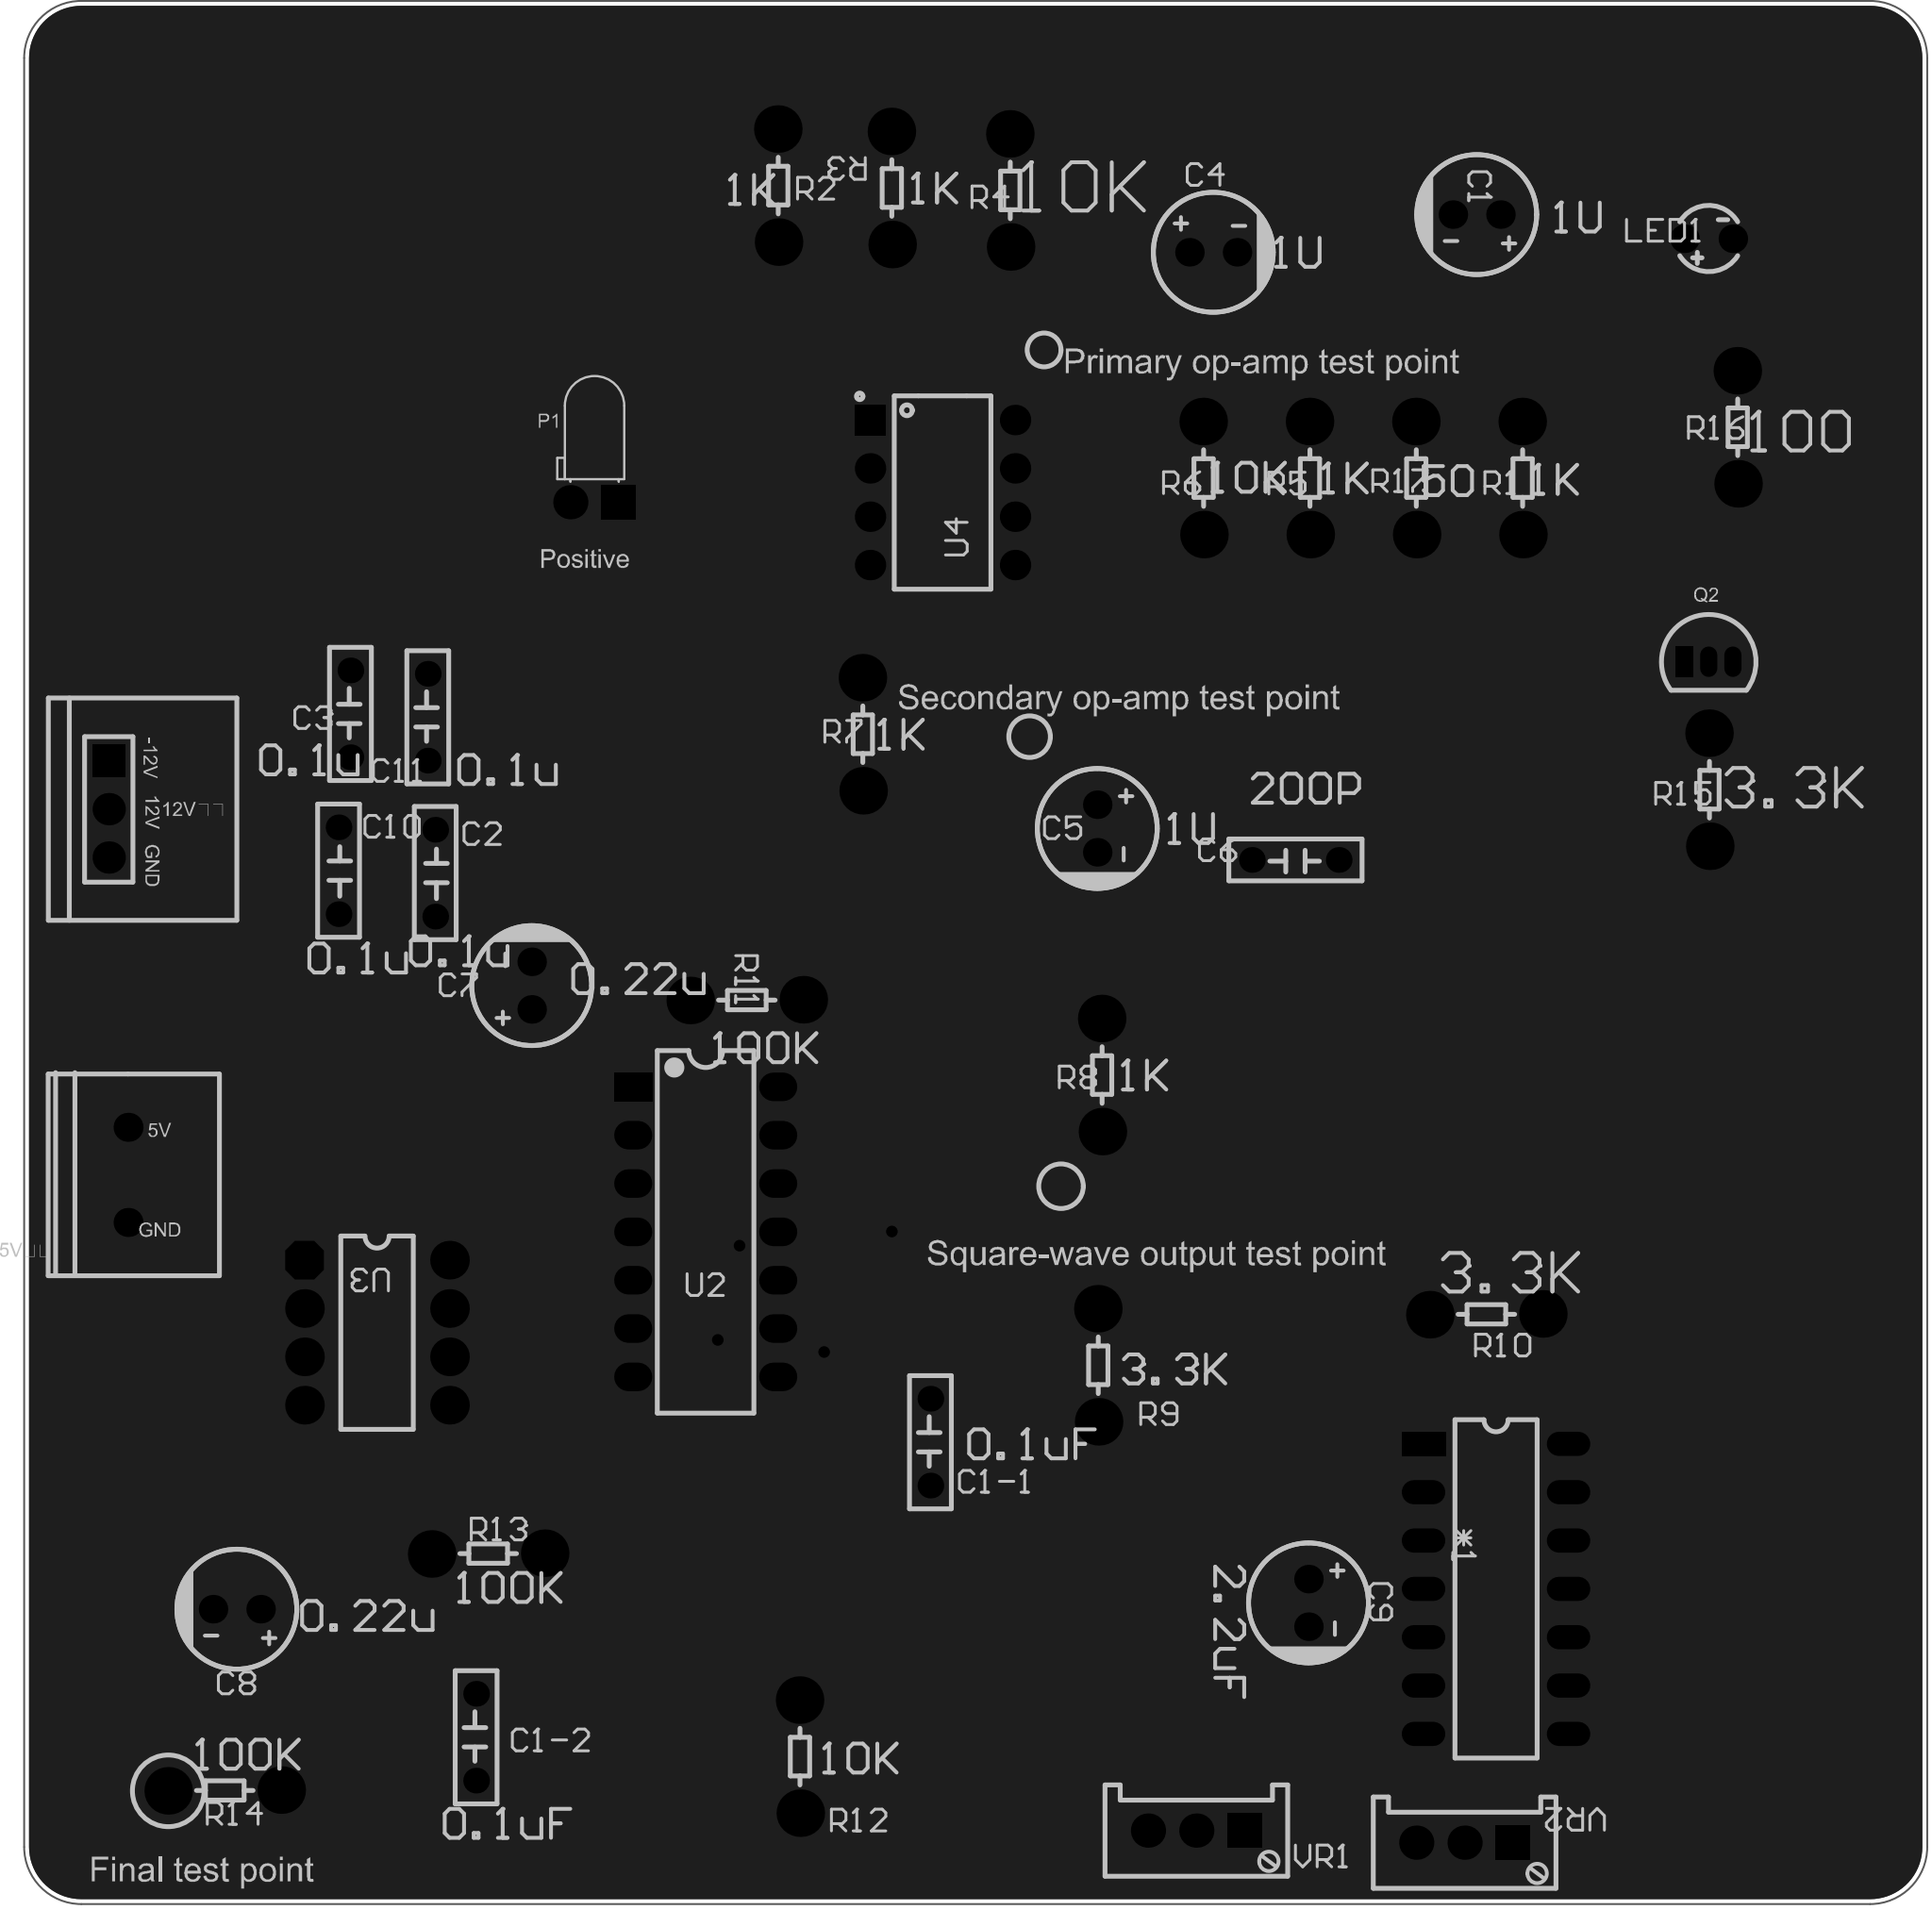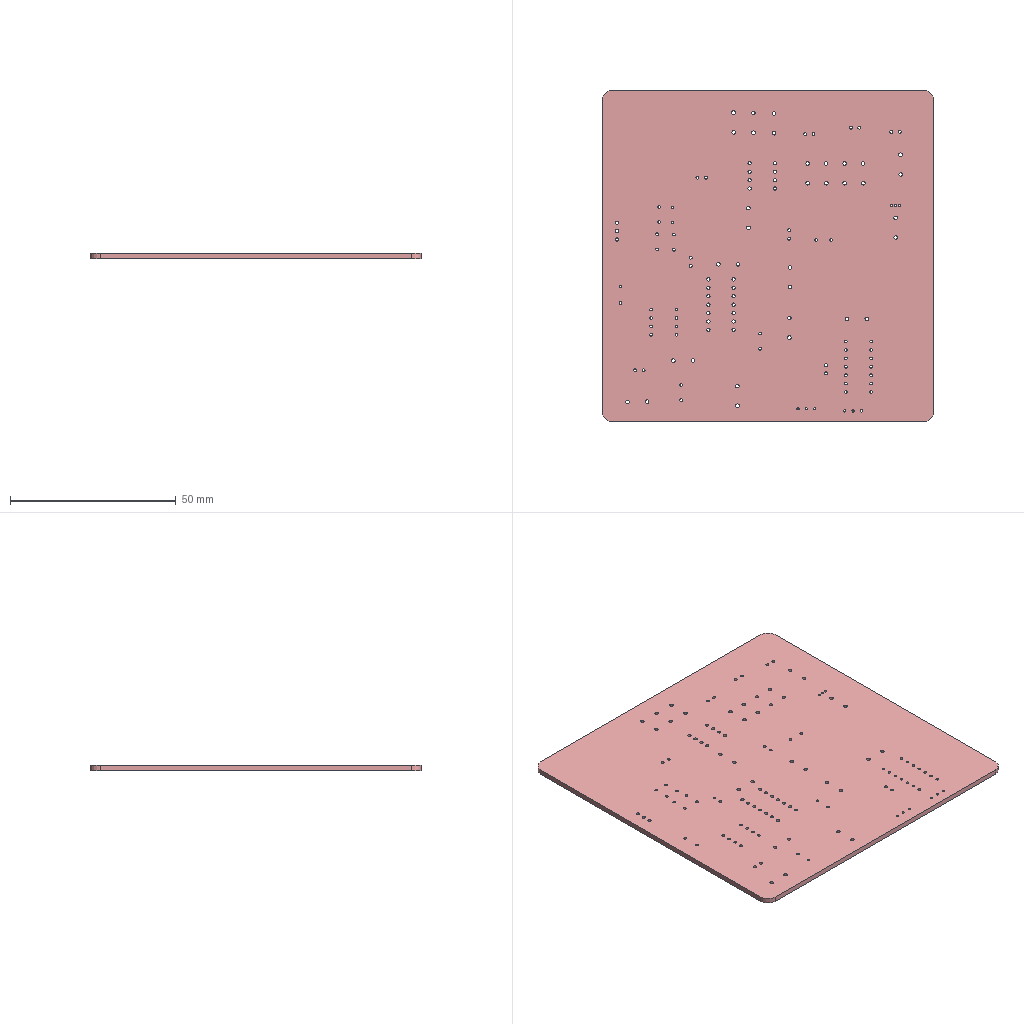Circuit board layout | Altium Designer | box 100 x 100 x 1.6 mm
Layer stack:
# Altium Designer layer stack of  (unit mm; dielectric type: 0 none, 1 core, 2 prepreg, 3 surface material)
index,name,kind,layer,copper_thickness_mm,dielectric_type,dielectric_thickness_mm,dielectric_material,dielectric_constant
0,Top Paste Mask Layer,other,,,,,,
1,Top Silkscreen Layer,other,,,,,,
2,Top Solder Mask Layer,dielectric,,,3,0.01,,3.3
3,Top Layer,copper,Top Layer,0.035,,,,
4,Dielectric1,dielectric,,,3,1.51,FR4,4.5
5,Bottom Layer,copper,Bottom Layer,0.035,,,,
6,Bottom Solder Mask Layer,dielectric,,,3,0.01,,3.3
7,Bottom Silkscreen Layer,other,,,,,,
8,Bottom Paste Mask Layer,other,,,,,,
# drill layer pairs: low layer,high layer
drill_pair,Top Layer,Bottom Layer
Part placement:
Designator,Comment,Layer,Footprint,Center-X(mm),Center-Y(mm),Rotation
C2,,TopLayer,电容直插,103.77,135.905,90
C3,,TopLayer,电容直插,99.314,144.277,270
P1,,TopLayer,LED_D3.0mm_Horizontal_O1.27mm_Z2.0mm,112.141,155.397,180
R1,,TopLayer,D45-V(直插),160.909,156.667,270
R2,,TopLayer,D45-V(直插),121.793,172.034,90
R3,,TopLayer,D45-V(直插),127.762,171.907,90
R4,,TopLayer,D45-V(直插),133.985,171.78,90
R5,,TopLayer,D45-V(直插),149.733,156.667,90
R6,,TopLayer,D45-V(直插),144.145,156.667,90
R7,,TopLayer,D45-V(直插),126.238,143.205,90
C6,,TopLayer,电容直插,148.966,136.601,0
U2,CD4066DN,TopLayer,PDIP-14_L19.3-W6.5-P2.54-LS7.6-BL,117.983,117.057,270
*1,74HC04,TopLayer,DIP14,159.512,98.298,0
C1,220uF,TopLayer,CAP-TH_BD6.3-P2.50-D0.5-FD,158.496,170.51,180
C1-1,,TopLayer,电容直插,129.79,106.007,270
C4,220uF,TopLayer,CAP-TH_BD6.3-P2.50-D0.5-FD,144.653,168.529,0
C5,220uF,TopLayer,CAP-TH_BD6.3-P2.50-D0.5-FD,138.557,138.252,270
C7,220uF,TopLayer,CAP-TH_BD6.3-P2.50-D0.5-FD,108.839,129.997,90
C8,220uF,TopLayer,CAP-TH_BD6.3-P2.50-D0.5-FD,93.345,97.231,180
C1-2,,TopLayer,电容直插,105.918,90.505,270
C10,,TopLayer,电容直插,98.69,136.032,90
C11,,TopLayer,电容直插,103.378,144.099,270
R8,,TopLayer,D45-V(直插),138.811,125.298,90
R9,,TopLayer,D45-V(直插),138.61,110.047,270
R10,,TopLayer,D45-V(直插),159.004,112.725,180
R11,,TopLayer,D45-V(直插),120.142,129.235,180
R12,,TopLayer,D45-V(直插),122.936,89.484,90
R13,,TopLayer,D45-V(直插),106.553,100.152,0
R14,,TopLayer,D45-V(直插),92.71,87.706,180
U3,LF353,TopLayer,DIP-8,100.711,111.76,0
5V输入,5V output,TopLayer,2INT,87.63,120.051,90
12V电源,3PIN,TopLayer,3PIN,86.614,139.268,90
C9,220uF,TopLayer,CAP-TH_BD6.3-P2.50-D0.5-FD,149.656,97.562,270
LED1,3A4GUD,TopLayer,LED-TH_BD3.5-P2.54-RD-GREEN,170.688,169.24,180
Q2,S9018,TopLayer,TO-92-3_L4.9-W3.7-P1.27-L,170.688,147.015,0
R15,,TopLayer,D45-V(直插),170.725,140.29,90
R16,,TopLayer,D45-V(直插),172.212,159.334,90
R17,,TopLayer,D45-V(直插),155.321,156.667,270
U4,,TopLayer,DIP-8_L9.9-W6.4-P2.54-LS7.6-BL,130.429,155.905,270
VR1,101,TopLayer,3296W,143.764,85.598,180
VR2,101,TopLayer,3296W,157.861,84.963,180
Pad and via stacks:
# Altium Designer via and pad stacks of  (unit mm). Each distinct definition once, with the count of objects using it.
# via: kind,start_layer,end_layer,hole_mm,diameter_mm,mode(0 simple;1 top-mid-bottom;2 full stack),diameter_per_layer,count,example_net
# pad: kind,layer,hole_mm,hole_type(0 round;1 square;2 slot),plating,top_size,top_shape(1 round;2 rect;3 octagon;9 rounded rect),mid_size,bottom_size,mode,footprint,size_per_layer,count,example
pad,Multi-Layer,0.81,0,plated,1.35x1.35,1,1.35x1.35,1.35x1.35,0,\u00B5\u00E7\u00C8\u00DD\u00D6\u00B1\u00B2\u00E5,,14,C2.1
pad,Multi-Layer,0.9,0,plated,1.8x1.8,2,1.8x1.8,1.8x1.8,0,LED_D3.0mm_Horizontal_O1.27mm_Z2.0mm,,1,P1.1
pad,Multi-Layer,0.9,0,plated,1.8x1.8,1,1.8x1.8,1.8x1.8,0,LED_D3.0mm_Horizontal_O1.27mm_Z2.0mm,,1,P1.2
pad,Multi-Layer,1.1,2,plated,2.5x2.5,1,2.5x2.5,2.5x2.5,0,D45-V(\u00D6\u00B1\u00B2\u00E5),,34,R1.2
pad,Multi-Layer,1,0,plated,1.5x2,1,1.5x2,1.5x2,0,PDIP-14_L19.3-W6.5-P2.54-LS7.6-BL,,13,U2.8
pad,Multi-Layer,1,0,plated,1.5x2,2,1.5x2,1.5x2,0,PDIP-14_L19.3-W6.5-P2.54-LS7.6-BL,,1,U2.1
pad,Multi-Layer,0.8128,0,plated,2.286x1.27,1,2.286x1.27,2.286x1.27,0,DIP14,,13,*1.8
pad,Multi-Layer,0.8128,0,plated,2.286x1.27,2,2.286x1.27,2.286x1.27,0,DIP14,,1,*1.1
pad,Multi-Layer,0.9,0,plated,1.5x1.5,1,1.5x1.5,1.5x1.5,0,CAP-TH_BD6.3-P2.50-D0.5-FD,,12,C1.2
pad,Multi-Layer,0.8128,0,plated,2.032x2.032,3,2.032x2.032,2.032x2.032,0,DIP-8,,1,U3.1
pad,Multi-Layer,0.8128,0,plated,2.032x2.032,1,1.27x1.27,2.032x2.032,1,DIP-8,,7,U3.2
pad,Multi-Layer,0.762,0,plated,1.524x1.524,1,1.524x1.524,1.524x1.524,0,2INT,,2,5V\u8F93\u5165.1
pad,Multi-Layer,1,0,plated,1.7x1.7,2,1.7x1.7,1.7x1.7,0,3PIN,,1,12V\u7535\u6E90.1
pad,Multi-Layer,1,0,plated,1.7x1.7,1,1.7x1.7,1.7x1.7,0,3PIN,,2,12V\u7535\u6E90.2
pad,Multi-Layer,0.9,0,plated,1.5x1.5,1,1.5x1.5,1.5x1.5,0,LED-TH_BD3.5-P2.54-RD-GREEN,,2,LED1.1
pad,Multi-Layer,0.7,0,plated,0.9x1.6,1,0.9x1.6,0.9x1.6,0,TO-92-3_L4.9-W3.7-P1.27-L,,2,Q2.3
pad,Multi-Layer,0.7,0,plated,0.9x1.6,2,0.9x1.6,0.9x1.6,0,TO-92-3_L4.9-W3.7-P1.27-L,,1,Q2.1
pad,Multi-Layer,1,0,plated,1.6x1.6,1,1.6x1.6,1.6x1.6,0,DIP-8_L9.9-W6.4-P2.54-LS7.6-BL,,7,U4.8
pad,Multi-Layer,1,0,plated,1.6x1.6,2,1.6x1.6,1.6x1.6,0,DIP-8_L9.9-W6.4-P2.54-LS7.6-BL,,1,U4.1
pad,Multi-Layer,0.7,0,plated,1.8x1.8,1,1.8x1.8,1.8x1.8,0,3296W,,4,VR1.3
pad,Multi-Layer,0.7,0,plated,1.8x1.8,2,1.8x1.8,1.8x1.8,0,3296W,,2,VR1.1
via,Top Layer,Bottom Layer,0.3048,0.61,0,,4,GND
Copper pours:
name,layer,net,type(0 solid;1 hatched;2 none)
Top Layer-GND,Top Layer,GND,0
Bottom Layer-GND,Bottom Layer,GND,0
Design rules, without the lines most boards share:
# Altium Designer design rules of  (exported by Altium Designer, unit mm)
# columns: name | kind | enabled | priority | scope1 | scope2 | descriptor | typed fields (field=value)
copperRegion | 20 | enabled | 1 | All | All | Polygon Connect Rule(Direct Connect )(Conductor Width=10mil) (Relief Angle=90 Angle) (Entries=4) (Air Gap Width=10mil) (All),(All) | connect_style(0=relief,1=direct,2=none)=1 relief_conductor_width=0.254 relief_entries=4
solderMaskExpansion | 13 | enabled | 2 | All | All | Solder Mask Expansion (Expansion =2.008mil) (All) | expansion=0.051